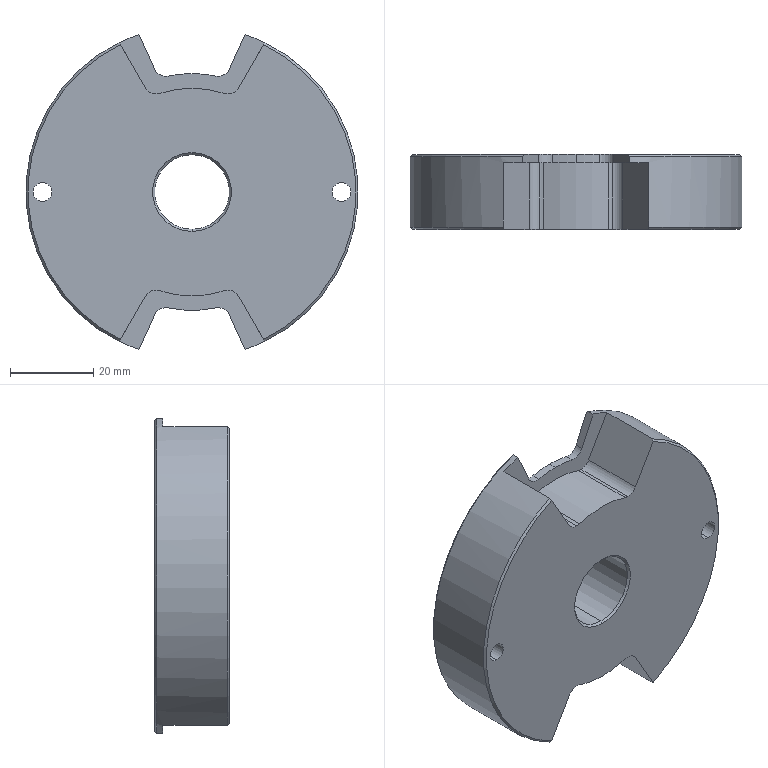Part | SolidWorks | features ICE 6, Chamfer 2, Extrusion 1 | 1 solid | 64 faces | box 80 x 18 x 75.795 mm | volume 68506 mm3 | cylinder 40 | plane 16 | cone 8 | commonest cylinder face diameters 6 x18 4.5 x4 50 x3 57 x3 18 x2 29 x2